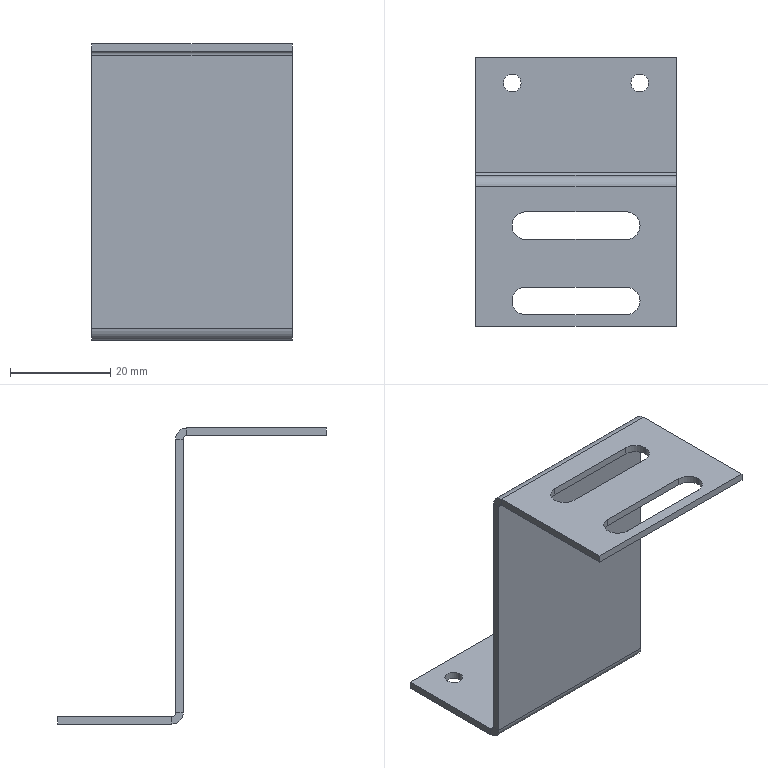Part | SolidWorks | features EdgeFlange 2, FlatPattern 1, ICE 1, SMBaseFlange 1, SheetMetal 1 | 1 solid | 36 faces | box 40 x 53.5 x 59 mm | volume 6153 mm3 | plane 22 | cylinder 14 | commonest cylinder face diameters 5.5 x6 3.5 x4 1.473 x2 4.473 x2
STEP:
#1=CARTESIAN_POINT('',(-14.45,33.5,-57.5));
#2=VERTEX_POINT('',#1);
#3=CARTESIAN_POINT('',(-10.95,33.5,-57.5));
#4=VERTEX_POINT('',#3);
#5=CARTESIAN_POINT('',(-12.7,33.5,-57.5));
#6=DIRECTION('',(0.,0.,1.));
#7=DIRECTION('',(1.,0.,0.));
#8=AXIS2_PLACEMENT_3D('',#5,#6,#7);
#9=CIRCLE('',#8,1.75);
#10=EDGE_CURVE('',#2,#4,#9,.T.);
#11=ORIENTED_EDGE('',*,*,#10,.T.);
#12=CARTESIAN_POINT('',(-10.95,33.5,-59.));
#13=VERTEX_POINT('',#12);
#14=CARTESIAN_POINT('',(-10.95,33.5,-49.));
#15=DIRECTION('',(0.,0.,-1.));
#16=VECTOR('',#15,1000.);
#17=LINE('',#14,#16);
#18=EDGE_CURVE('',#4,#13,#17,.T.);
#19=ORIENTED_EDGE('',*,*,#18,.T.);
#20=CARTESIAN_POINT('',(-14.45,33.5,-59.));
#21=VERTEX_POINT('',#20);
#22=CARTESIAN_POINT('',(-12.7,33.5,-59.));
#23=DIRECTION('',(0.,0.,-1.));
#24=DIRECTION('',(-1.,0.,0.));
#25=AXIS2_PLACEMENT_3D('',#22,#23,#24);
#26=CIRCLE('',#25,1.75);
#27=EDGE_CURVE('',#13,#21,#26,.T.);
#28=ORIENTED_EDGE('',*,*,#27,.T.);
#29=CARTESIAN_POINT('',(-14.45,33.5,-49.));
#30=DIRECTION('',(0.,0.,-1.));
#31=VECTOR('',#30,1000.);
#32=LINE('',#29,#31);
#33=EDGE_CURVE('',#2,#21,#32,.T.);
#34=ORIENTED_EDGE('',*,*,#33,.F.);
#35=EDGE_LOOP('',(#11,#19,#28,#34));
#36=FACE_OUTER_BOUND('',#35,.T.);
#37=CARTESIAN_POINT('',(-12.7,33.5,-49.));
#38=DIRECTION('',(0.,0.,-1.));
#39=DIRECTION('',(-1.,0.,0.));
#40=AXIS2_PLACEMENT_3D('',#37,#38,#39);
#41=CYLINDRICAL_SURFACE('',#40,1.75);
#42=ADVANCED_FACE('',(#36),#41,.F.);
#43=CARTESIAN_POINT('',(10.95,33.5,-57.5));
#44=VERTEX_POINT('',#43);
#45=CARTESIAN_POINT('',(14.45,33.5,-57.5));
#46=VERTEX_POINT('',#45);
#47=CARTESIAN_POINT('',(12.7,33.5,-57.5));
#48=DIRECTION('',(0.,0.,1.));
#49=DIRECTION('',(1.,0.,0.));
#50=AXIS2_PLACEMENT_3D('',#47,#48,#49);
#51=CIRCLE('',#50,1.75);
#52=EDGE_CURVE('',#44,#46,#51,.T.);
#53=ORIENTED_EDGE('',*,*,#52,.T.);
#54=CARTESIAN_POINT('',(14.45,33.5,-59.));
#55=VERTEX_POINT('',#54);
#56=CARTESIAN_POINT('',(14.45,33.5,-49.));
#57=DIRECTION('',(0.,0.,-1.));
#58=VECTOR('',#57,1000.);
#59=LINE('',#56,#58);
#60=EDGE_CURVE('',#46,#55,#59,.T.);
#61=ORIENTED_EDGE('',*,*,#60,.T.);
#62=CARTESIAN_POINT('',(10.95,33.5,-59.));
#63=VERTEX_POINT('',#62);
#64=CARTESIAN_POINT('',(12.7,33.5,-59.));
#65=DIRECTION('',(0.,0.,-1.));
#66=DIRECTION('',(-1.,0.,0.));
#67=AXIS2_PLACEMENT_3D('',#64,#65,#66);
#68=CIRCLE('',#67,1.75);
#69=EDGE_CURVE('',#55,#63,#68,.T.);
#70=ORIENTED_EDGE('',*,*,#69,.T.);
#71=CARTESIAN_POINT('',(10.95,33.5,-49.));
#72=DIRECTION('',(0.,0.,-1.));
#73=VECTOR('',#72,1000.);
#74=LINE('',#71,#73);
#75=EDGE_CURVE('',#44,#63,#74,.T.);
#76=ORIENTED_EDGE('',*,*,#75,.F.);
#77=EDGE_LOOP('',(#53,#61,#70,#76));
#78=FACE_OUTER_BOUND('',#77,.T.);
#79=CARTESIAN_POINT('',(12.7,33.5,-49.));
#80=DIRECTION('',(0.,0.,-1.));
#81=DIRECTION('',(-1.,0.,0.));
#82=AXIS2_PLACEMENT_3D('',#79,#80,#81);
#83=CYLINDRICAL_SURFACE('',#82,1.75);
#84=ADVANCED_FACE('',(#78),#83,.F.);
#85=CARTESIAN_POINT('',(12.75,-10.,-1.5));
#86=VERTEX_POINT('',#85);
#87=CARTESIAN_POINT('',(10.,-7.25,-1.5));
#88=VERTEX_POINT('',#87);
#89=CARTESIAN_POINT('',(10.,-10.,-1.5));
#90=DIRECTION('',(0.,0.,1.));
#91=DIRECTION('',(1.,0.,0.));
#92=AXIS2_PLACEMENT_3D('',#89,#90,#91);
#93=CIRCLE('',#92,2.75);
#94=EDGE_CURVE('',#86,#88,#93,.T.);
#95=ORIENTED_EDGE('',*,*,#94,.F.);
#96=CARTESIAN_POINT('',(12.75,-10.,0.));
#97=VERTEX_POINT('',#96);
#98=CARTESIAN_POINT('',(12.75,-10.,-1.5));
#99=DIRECTION('',(0.,0.,1.));
#100=VECTOR('',#99,1000.);
#101=LINE('',#98,#100);
#102=EDGE_CURVE('',#86,#97,#101,.T.);
#103=ORIENTED_EDGE('',*,*,#102,.T.);
#104=CARTESIAN_POINT('',(10.,-7.25,0.));
#105=VERTEX_POINT('',#104);
#106=CARTESIAN_POINT('',(10.,-10.,0.));
#107=DIRECTION('',(0.,0.,1.));
#108=DIRECTION('',(1.,0.,0.));
#109=AXIS2_PLACEMENT_3D('',#106,#107,#108);
#110=CIRCLE('',#109,2.75);
#111=EDGE_CURVE('',#97,#105,#110,.T.);
#112=ORIENTED_EDGE('',*,*,#111,.T.);
#113=CARTESIAN_POINT('',(10.,-7.25,-1.5));
#114=DIRECTION('',(0.,0.,1.));
#115=VECTOR('',#114,1000.);
#116=LINE('',#113,#115);
#117=EDGE_CURVE('',#88,#105,#116,.T.);
#118=ORIENTED_EDGE('',*,*,#117,.F.);
#119=EDGE_LOOP('',(#95,#103,#112,#118));
#120=FACE_OUTER_BOUND('',#119,.T.);
#121=CARTESIAN_POINT('',(10.,-10.,-1.5));
#122=DIRECTION('',(0.,0.,1.));
#123=DIRECTION('',(1.,0.,0.));
#124=AXIS2_PLACEMENT_3D('',#121,#122,#123);
#125=CYLINDRICAL_SURFACE('',#124,2.75);
#126=ADVANCED_FACE('',(#120),#125,.F.);
#127=CARTESIAN_POINT('',(12.75,5.,-1.5));
#128=VERTEX_POINT('',#127);
#129=CARTESIAN_POINT('',(10.,7.75,-1.5));
#130=VERTEX_POINT('',#129);
#131=CARTESIAN_POINT('',(10.,5.,-1.5));
#132=DIRECTION('',(0.,0.,1.));
#133=DIRECTION('',(1.,0.,0.));
#134=AXIS2_PLACEMENT_3D('',#131,#132,#133);
#135=CIRCLE('',#134,2.75);
#136=EDGE_CURVE('',#128,#130,#135,.T.);
#137=ORIENTED_EDGE('',*,*,#136,.F.);
#138=CARTESIAN_POINT('',(12.75,5.,0.));
#139=VERTEX_POINT('',#138);
#140=CARTESIAN_POINT('',(12.75,5.,-1.5));
#141=DIRECTION('',(0.,0.,1.));
#142=VECTOR('',#141,1000.);
#143=LINE('',#140,#142);
#144=EDGE_CURVE('',#128,#139,#143,.T.);
#145=ORIENTED_EDGE('',*,*,#144,.T.);
#146=CARTESIAN_POINT('',(10.,7.75,0.));
#147=VERTEX_POINT('',#146);
#148=CARTESIAN_POINT('',(10.,5.,0.));
#149=DIRECTION('',(0.,0.,1.));
#150=DIRECTION('',(1.,0.,0.));
#151=AXIS2_PLACEMENT_3D('',#148,#149,#150);
#152=CIRCLE('',#151,2.75);
#153=EDGE_CURVE('',#139,#147,#152,.T.);
#154=ORIENTED_EDGE('',*,*,#153,.T.);
#155=CARTESIAN_POINT('',(10.,7.75,-1.5));
#156=DIRECTION('',(0.,0.,1.));
#157=VECTOR('',#156,1000.);
#158=LINE('',#155,#157);
#159=EDGE_CURVE('',#130,#147,#158,.T.);
#160=ORIENTED_EDGE('',*,*,#159,.F.);
#161=EDGE_LOOP('',(#137,#145,#154,#160));
#162=FACE_OUTER_BOUND('',#161,.T.);
#163=CARTESIAN_POINT('',(10.,5.,-1.5));
#164=DIRECTION('',(0.,0.,1.));
#165=DIRECTION('',(1.,0.,0.));
#166=AXIS2_PLACEMENT_3D('',#163,#164,#165);
#167=CYLINDRICAL_SURFACE('',#166,2.75);
#168=ADVANCED_FACE('',(#162),#167,.F.);
#169=CARTESIAN_POINT('',(-20.,15.,-2.237));
#170=VERTEX_POINT('',#169);
#171=CARTESIAN_POINT('',(-20.,15.,-56.763));
#172=VERTEX_POINT('',#171);
#173=CARTESIAN_POINT('',(-20.,15.,-59.));
#174=DIRECTION('',(0.,0.,-1.));
#175=VECTOR('',#174,1000.);
#176=LINE('',#173,#175);
#177=EDGE_CURVE('',#170,#172,#176,.T.);
#178=ORIENTED_EDGE('',*,*,#177,.T.);
#179=CARTESIAN_POINT('',(-20.,13.5,-56.763));
#180=VERTEX_POINT('',#179);
#181=CARTESIAN_POINT('',(-20.,15.,-56.763));
#182=DIRECTION('',(0.,-1.,0.));
#183=VECTOR('',#182,1000.);
#184=LINE('',#181,#183);
#185=EDGE_CURVE('',#172,#180,#184,.T.);
#186=ORIENTED_EDGE('',*,*,#185,.T.);
#187=CARTESIAN_POINT('',(-20.,13.5,-2.237));
#188=VERTEX_POINT('',#187);
#189=CARTESIAN_POINT('',(-20.,13.5,0.));
#190=DIRECTION('',(0.,0.,-1.));
#191=VECTOR('',#190,1000.);
#192=LINE('',#189,#191);
#193=EDGE_CURVE('',#188,#180,#192,.T.);
#194=ORIENTED_EDGE('',*,*,#193,.F.);
#195=CARTESIAN_POINT('',(-20.,15.,-2.237));
#196=DIRECTION('',(0.,1.,0.));
#197=VECTOR('',#196,1000.);
#198=LINE('',#195,#197);
#199=EDGE_CURVE('',#188,#170,#198,.T.);
#200=ORIENTED_EDGE('',*,*,#199,.T.);
#201=EDGE_LOOP('',(#178,#186,#194,#200));
#202=FACE_OUTER_BOUND('',#201,.T.);
#203=CARTESIAN_POINT('',(-20.,15.,-59.));
#204=DIRECTION('',(-1.,0.,0.));
#205=DIRECTION('',(0.,0.,1.));
#206=AXIS2_PLACEMENT_3D('',#203,#204,#205);
#207=PLANE('',#206);
#208=ADVANCED_FACE('',(#202),#207,.T.);
#209=CARTESIAN_POINT('',(20.,15.,-56.763));
#210=VERTEX_POINT('',#209);
#211=CARTESIAN_POINT('',(20.,15.,-2.237));
#212=VERTEX_POINT('',#211);
#213=CARTESIAN_POINT('',(20.,15.,-1.5));
#214=DIRECTION('',(0.,0.,1.));
#215=VECTOR('',#214,1000.);
#216=LINE('',#213,#215);
#217=EDGE_CURVE('',#210,#212,#216,.T.);
#218=ORIENTED_EDGE('',*,*,#217,.F.);
#219=CARTESIAN_POINT('',(-20.,15.,-56.763));
#220=DIRECTION('',(1.,0.,0.));
#221=VECTOR('',#220,1000.);
#222=LINE('',#219,#221);
#223=EDGE_CURVE('',#172,#210,#222,.T.);
#224=ORIENTED_EDGE('',*,*,#223,.F.);
#225=ORIENTED_EDGE('',*,*,#177,.F.);
#226=CARTESIAN_POINT('',(0.,15.,-2.237));
#227=DIRECTION('',(1.,0.,0.));
#228=VECTOR('',#227,1000.);
#229=LINE('',#226,#228);
#230=EDGE_CURVE('',#170,#212,#229,.T.);
#231=ORIENTED_EDGE('',*,*,#230,.T.);
#232=EDGE_LOOP('',(#218,#224,#225,#231));
#233=FACE_OUTER_BOUND('',#232,.T.);
#234=CARTESIAN_POINT('',(0.,15.,0.));
#235=DIRECTION('',(0.,1.,0.));
#236=DIRECTION('',(0.,0.,1.));
#237=AXIS2_PLACEMENT_3D('',#234,#235,#236);
#238=PLANE('',#237);
#239=ADVANCED_FACE('',(#233),#238,.T.);
#240=CARTESIAN_POINT('',(20.,13.5,-56.763));
#241=VERTEX_POINT('',#240);
#242=CARTESIAN_POINT('',(-20.,13.5,-56.763));
#243=DIRECTION('',(1.,0.,0.));
#244=VECTOR('',#243,1000.);
#245=LINE('',#242,#244);
#246=EDGE_CURVE('',#180,#241,#245,.T.);
#247=ORIENTED_EDGE('',*,*,#246,.T.);
#248=CARTESIAN_POINT('',(20.,13.5,-2.237));
#249=VERTEX_POINT('',#248);
#250=CARTESIAN_POINT('',(20.,13.5,0.));
#251=DIRECTION('',(0.,0.,1.));
#252=VECTOR('',#251,1000.);
#253=LINE('',#250,#252);
#254=EDGE_CURVE('',#241,#249,#253,.T.);
#255=ORIENTED_EDGE('',*,*,#254,.T.);
#256=CARTESIAN_POINT('',(-20.,13.5,-2.237));
#257=DIRECTION('',(1.,0.,0.));
#258=VECTOR('',#257,1000.);
#259=LINE('',#256,#258);
#260=EDGE_CURVE('',#188,#249,#259,.T.);
#261=ORIENTED_EDGE('',*,*,#260,.F.);
#262=ORIENTED_EDGE('',*,*,#193,.T.);
#263=EDGE_LOOP('',(#247,#255,#261,#262));
#264=FACE_OUTER_BOUND('',#263,.T.);
#265=CARTESIAN_POINT('',(0.,13.5,0.));
#266=DIRECTION('',(0.,1.,0.));
#267=DIRECTION('',(0.,0.,1.));
#268=AXIS2_PLACEMENT_3D('',#265,#266,#267);
#269=PLANE('',#268);
#270=ADVANCED_FACE('',(#264),#269,.F.);
#271=CARTESIAN_POINT('',(20.,-15.,-1.5));
#272=VERTEX_POINT('',#271);
#273=CARTESIAN_POINT('',(20.,12.763,-1.5));
#274=VERTEX_POINT('',#273);
#275=CARTESIAN_POINT('',(20.,15.,-1.5));
#276=DIRECTION('',(0.,1.,0.));
#277=VECTOR('',#276,1000.);
#278=LINE('',#275,#277);
#279=EDGE_CURVE('',#272,#274,#278,.T.);
#280=ORIENTED_EDGE('',*,*,#279,.T.);
#281=CARTESIAN_POINT('',(20.,12.763,0.));
#282=VERTEX_POINT('',#281);
#283=CARTESIAN_POINT('',(20.,12.763,-1.5));
#284=DIRECTION('',(0.,0.,1.));
#285=VECTOR('',#284,1000.);
#286=LINE('',#283,#285);
#287=EDGE_CURVE('',#274,#282,#286,.T.);
#288=ORIENTED_EDGE('',*,*,#287,.T.);
#289=CARTESIAN_POINT('',(20.,-15.,0.));
#290=VERTEX_POINT('',#289);
#291=CARTESIAN_POINT('',(20.,15.,0.));
#292=DIRECTION('',(0.,1.,0.));
#293=VECTOR('',#292,1000.);
#294=LINE('',#291,#293);
#295=EDGE_CURVE('',#290,#282,#294,.T.);
#296=ORIENTED_EDGE('',*,*,#295,.F.);
#297=CARTESIAN_POINT('',(20.,-15.,-1.5));
#298=DIRECTION('',(0.,0.,1.));
#299=VECTOR('',#298,1000.);
#300=LINE('',#297,#299);
#301=EDGE_CURVE('',#272,#290,#300,.T.);
#302=ORIENTED_EDGE('',*,*,#301,.F.);
#303=EDGE_LOOP('',(#280,#288,#296,#302));
#304=FACE_OUTER_BOUND('',#303,.T.);
#305=CARTESIAN_POINT('',(20.,15.,-1.5));
#306=DIRECTION('',(1.,0.,0.));
#307=DIRECTION('',(0.,0.,-1.));
#308=AXIS2_PLACEMENT_3D('',#305,#306,#307);
#309=PLANE('',#308);
#310=ADVANCED_FACE('',(#304),#309,.T.);
#311=CARTESIAN_POINT('',(-10.,2.25,-1.5));
#312=VERTEX_POINT('',#311);
#313=CARTESIAN_POINT('',(10.,2.25,-1.5));
#314=VERTEX_POINT('',#313);
#315=CARTESIAN_POINT('',(10.,2.25,-1.5));
#316=DIRECTION('',(1.,0.,0.));
#317=VECTOR('',#316,1000.);
#318=LINE('',#315,#317);
#319=EDGE_CURVE('',#312,#314,#318,.T.);
#320=ORIENTED_EDGE('',*,*,#319,.T.);
#321=CARTESIAN_POINT('',(10.,5.,-1.5));
#322=DIRECTION('',(0.,0.,1.));
#323=DIRECTION('',(1.,0.,0.));
#324=AXIS2_PLACEMENT_3D('',#321,#322,#323);
#325=CIRCLE('',#324,2.75);
#326=EDGE_CURVE('',#314,#128,#325,.T.);
#327=ORIENTED_EDGE('',*,*,#326,.T.);
#328=ORIENTED_EDGE('',*,*,#136,.T.);
#329=CARTESIAN_POINT('',(-10.,7.75,-1.5));
#330=VERTEX_POINT('',#329);
#331=CARTESIAN_POINT('',(10.,7.75,-1.5));
#332=DIRECTION('',(-1.,0.,0.));
#333=VECTOR('',#332,1000.);
#334=LINE('',#331,#333);
#335=EDGE_CURVE('',#130,#330,#334,.T.);
#336=ORIENTED_EDGE('',*,*,#335,.T.);
#337=CARTESIAN_POINT('',(-10.,5.,-1.5));
#338=DIRECTION('',(0.,0.,1.));
#339=DIRECTION('',(1.,0.,0.));
#340=AXIS2_PLACEMENT_3D('',#337,#338,#339);
#341=CIRCLE('',#340,2.75);
#342=EDGE_CURVE('',#330,#312,#341,.T.);
#343=ORIENTED_EDGE('',*,*,#342,.T.);
#344=EDGE_LOOP('',(#320,#327,#328,#336,#343));
#345=FACE_BOUND('',#344,.T.);
#346=CARTESIAN_POINT('',(-10.,-12.75,-1.5));
#347=VERTEX_POINT('',#346);
#348=CARTESIAN_POINT('',(10.,-12.75,-1.5));
#349=VERTEX_POINT('',#348);
#350=CARTESIAN_POINT('',(10.,-12.75,-1.5));
#351=DIRECTION('',(1.,0.,0.));
#352=VECTOR('',#351,1000.);
#353=LINE('',#350,#352);
#354=EDGE_CURVE('',#347,#349,#353,.T.);
#355=ORIENTED_EDGE('',*,*,#354,.T.);
#356=CARTESIAN_POINT('',(10.,-10.,-1.5));
#357=DIRECTION('',(0.,0.,1.));
#358=DIRECTION('',(1.,0.,0.));
#359=AXIS2_PLACEMENT_3D('',#356,#357,#358);
#360=CIRCLE('',#359,2.75);
#361=EDGE_CURVE('',#349,#86,#360,.T.);
#362=ORIENTED_EDGE('',*,*,#361,.T.);
#363=ORIENTED_EDGE('',*,*,#94,.T.);
#364=CARTESIAN_POINT('',(-10.,-7.25,-1.5));
#365=VERTEX_POINT('',#364);
#366=CARTESIAN_POINT('',(10.,-7.25,-1.5));
#367=DIRECTION('',(-1.,0.,0.));
#368=VECTOR('',#367,1000.);
#369=LINE('',#366,#368);
#370=EDGE_CURVE('',#88,#365,#369,.T.);
#371=ORIENTED_EDGE('',*,*,#370,.T.);
#372=CARTESIAN_POINT('',(-10.,-10.,-1.5));
#373=DIRECTION('',(0.,0.,1.));
#374=DIRECTION('',(1.,0.,0.));
#375=AXIS2_PLACEMENT_3D('',#372,#373,#374);
#376=CIRCLE('',#375,2.75);
#377=EDGE_CURVE('',#365,#347,#376,.T.);
#378=ORIENTED_EDGE('',*,*,#377,.T.);
#379=EDGE_LOOP('',(#355,#362,#363,#371,#378));
#380=FACE_BOUND('',#379,.T.);
#381=CARTESIAN_POINT('',(-20.,12.763,-1.5));
#382=VERTEX_POINT('',#381);
#383=CARTESIAN_POINT('',(20.,12.763,-1.5));
#384=DIRECTION('',(-1.,0.,0.));
#385=VECTOR('',#384,1000.);
#386=LINE('',#383,#385);
#387=EDGE_CURVE('',#274,#382,#386,.T.);
#388=ORIENTED_EDGE('',*,*,#387,.F.);
#389=ORIENTED_EDGE('',*,*,#279,.F.);
#390=CARTESIAN_POINT('',(-20.,-15.,-1.5));
#391=VERTEX_POINT('',#390);
#392=CARTESIAN_POINT('',(-20.,-15.,-1.5));
#393=DIRECTION('',(1.,0.,0.));
#394=VECTOR('',#393,1000.);
#395=LINE('',#392,#394);
#396=EDGE_CURVE('',#391,#272,#395,.T.);
#397=ORIENTED_EDGE('',*,*,#396,.F.);
#398=CARTESIAN_POINT('',(-20.,15.,-1.5));
#399=DIRECTION('',(0.,-1.,0.));
#400=VECTOR('',#399,1000.);
#401=LINE('',#398,#400);
#402=EDGE_CURVE('',#382,#391,#401,.T.);
#403=ORIENTED_EDGE('',*,*,#402,.F.);
#404=EDGE_LOOP('',(#388,#389,#397,#403));
#405=FACE_OUTER_BOUND('',#404,.T.);
#406=CARTESIAN_POINT('',(0.,0.,-1.5));
#407=DIRECTION('',(0.,0.,1.));
#408=DIRECTION('',(1.,0.,0.));
#409=AXIS2_PLACEMENT_3D('',#406,#407,#408);
#410=PLANE('',#409);
#411=ADVANCED_FACE('',(#345,#380,#405),#410,.F.);
#412=CARTESIAN_POINT('',(10.,2.25,0.));
#413=VERTEX_POINT('',#412);
#414=CARTESIAN_POINT('',(10.,5.,0.));
#415=DIRECTION('',(0.,0.,1.));
#416=DIRECTION('',(1.,0.,0.));
#417=AXIS2_PLACEMENT_3D('',#414,#415,#416);
#418=CIRCLE('',#417,2.75);
#419=EDGE_CURVE('',#413,#139,#418,.T.);
#420=ORIENTED_EDGE('',*,*,#419,.F.);
#421=CARTESIAN_POINT('',(-10.,2.25,0.));
#422=VERTEX_POINT('',#421);
#423=CARTESIAN_POINT('',(10.,2.25,0.));
#424=DIRECTION('',(1.,0.,0.));
#425=VECTOR('',#424,1000.);
#426=LINE('',#423,#425);
#427=EDGE_CURVE('',#422,#413,#426,.T.);
#428=ORIENTED_EDGE('',*,*,#427,.F.);
#429=CARTESIAN_POINT('',(-10.,7.75,0.));
#430=VERTEX_POINT('',#429);
#431=CARTESIAN_POINT('',(-10.,5.,0.));
#432=DIRECTION('',(0.,0.,1.));
#433=DIRECTION('',(1.,0.,0.));
#434=AXIS2_PLACEMENT_3D('',#431,#432,#433);
#435=CIRCLE('',#434,2.75);
#436=EDGE_CURVE('',#430,#422,#435,.T.);
#437=ORIENTED_EDGE('',*,*,#436,.F.);
#438=CARTESIAN_POINT('',(10.,7.75,0.));
#439=DIRECTION('',(-1.,0.,0.));
#440=VECTOR('',#439,1000.);
#441=LINE('',#438,#440);
#442=EDGE_CURVE('',#147,#430,#441,.T.);
#443=ORIENTED_EDGE('',*,*,#442,.F.);
#444=ORIENTED_EDGE('',*,*,#153,.F.);
#445=EDGE_LOOP('',(#420,#428,#437,#443,#444));
#446=FACE_BOUND('',#445,.T.);
#447=CARTESIAN_POINT('',(10.,-12.75,0.));
#448=VERTEX_POINT('',#447);
#449=CARTESIAN_POINT('',(10.,-10.,0.));
#450=DIRECTION('',(0.,0.,1.));
#451=DIRECTION('',(1.,0.,0.));
#452=AXIS2_PLACEMENT_3D('',#449,#450,#451);
#453=CIRCLE('',#452,2.75);
#454=EDGE_CURVE('',#448,#97,#453,.T.);
#455=ORIENTED_EDGE('',*,*,#454,.F.);
#456=CARTESIAN_POINT('',(-10.,-12.75,0.));
#457=VERTEX_POINT('',#456);
#458=CARTESIAN_POINT('',(10.,-12.75,0.));
#459=DIRECTION('',(1.,0.,0.));
#460=VECTOR('',#459,1000.);
#461=LINE('',#458,#460);
#462=EDGE_CURVE('',#457,#448,#461,.T.);
#463=ORIENTED_EDGE('',*,*,#462,.F.);
#464=CARTESIAN_POINT('',(-10.,-7.25,0.));
#465=VERTEX_POINT('',#464);
#466=CARTESIAN_POINT('',(-10.,-10.,0.));
#467=DIRECTION('',(0.,0.,1.));
#468=DIRECTION('',(1.,0.,0.));
#469=AXIS2_PLACEMENT_3D('',#466,#467,#468);
#470=CIRCLE('',#469,2.75);
#471=EDGE_CURVE('',#465,#457,#470,.T.);
#472=ORIENTED_EDGE('',*,*,#471,.F.);
#473=CARTESIAN_POINT('',(10.,-7.25,0.));
#474=DIRECTION('',(-1.,0.,0.));
#475=VECTOR('',#474,1000.);
#476=LINE('',#473,#475);
#477=EDGE_CURVE('',#105,#465,#476,.T.);
#478=ORIENTED_EDGE('',*,*,#477,.F.);
#479=ORIENTED_EDGE('',*,*,#111,.F.);
#480=EDGE_LOOP('',(#455,#463,#472,#478,#479));
#481=FACE_BOUND('',#480,.T.);
#482=ORIENTED_EDGE('',*,*,#295,.T.);
#483=CARTESIAN_POINT('',(-20.,12.763,0.));
#484=VERTEX_POINT('',#483);
#485=CARTESIAN_POINT('',(20.,12.763,0.));
#486=DIRECTION('',(-1.,0.,0.));
#487=VECTOR('',#486,1000.);
#488=LINE('',#485,#487);
#489=EDGE_CURVE('',#282,#484,#488,.T.);
#490=ORIENTED_EDGE('',*,*,#489,.T.);
#491=CARTESIAN_POINT('',(-20.,-15.,0.));
#492=VERTEX_POINT('',#491);
#493=CARTESIAN_POINT('',(-20.,15.,0.));
#494=DIRECTION('',(0.,-1.,0.));
#495=VECTOR('',#494,1000.);
#496=LINE('',#493,#495);
#497=EDGE_CURVE('',#484,#492,#496,.T.);
#498=ORIENTED_EDGE('',*,*,#497,.T.);
#499=CARTESIAN_POINT('',(-20.,-15.,0.));
#500=DIRECTION('',(1.,0.,0.));
#501=VECTOR('',#500,1000.);
#502=LINE('',#499,#501);
#503=EDGE_CURVE('',#492,#290,#502,.T.);
#504=ORIENTED_EDGE('',*,*,#503,.T.);
#505=EDGE_LOOP('',(#482,#490,#498,#504));
#506=FACE_OUTER_BOUND('',#505,.T.);
#507=CARTESIAN_POINT('',(0.,0.,0.));
#508=DIRECTION('',(0.,0.,1.));
#509=DIRECTION('',(1.,0.,0.));
#510=AXIS2_PLACEMENT_3D('',#507,#508,#509);
#511=PLANE('',#510);
#512=ADVANCED_FACE('',(#446,#481,#506),#511,.T.);
#513=ORIENTED_EDGE('',*,*,#503,.F.);
#514=CARTESIAN_POINT('',(-20.,-15.,-1.5));
#515=DIRECTION('',(0.,0.,1.));
#516=VECTOR('',#515,1000.);
#517=LINE('',#514,#516);
#518=EDGE_CURVE('',#391,#492,#517,.T.);
#519=ORIENTED_EDGE('',*,*,#518,.F.);
#520=ORIENTED_EDGE('',*,*,#396,.T.);
#521=ORIENTED_EDGE('',*,*,#301,.T.);
#522=EDGE_LOOP('',(#513,#519,#520,#521));
#523=FACE_OUTER_BOUND('',#522,.T.);
#524=CARTESIAN_POINT('',(-20.,-15.,-1.5));
#525=DIRECTION('',(0.,-1.,0.));
#526=DIRECTION('',(0.,0.,-1.));
#527=AXIS2_PLACEMENT_3D('',#524,#525,#526);
#528=PLANE('',#527);
#529=ADVANCED_FACE('',(#523),#528,.T.);
#530=CARTESIAN_POINT('',(-20.,12.763,-1.5));
#531=DIRECTION('',(0.,0.,1.));
#532=VECTOR('',#531,1000.);
#533=LINE('',#530,#532);
#534=EDGE_CURVE('',#382,#484,#533,.T.);
#535=ORIENTED_EDGE('',*,*,#534,.F.);
#536=ORIENTED_EDGE('',*,*,#402,.T.);
#537=ORIENTED_EDGE('',*,*,#518,.T.);
#538=ORIENTED_EDGE('',*,*,#497,.F.);
#539=EDGE_LOOP('',(#535,#536,#537,#538));
#540=FACE_OUTER_BOUND('',#539,.T.);
#541=CARTESIAN_POINT('',(-20.,15.,-1.5));
#542=DIRECTION('',(-1.,0.,0.));
#543=DIRECTION('',(0.,0.,1.));
#544=AXIS2_PLACEMENT_3D('',#541,#542,#543);
#545=PLANE('',#544);
#546=ADVANCED_FACE('',(#540),#545,.T.);
#547=ORIENTED_EDGE('',*,*,#144,.F.);
#548=ORIENTED_EDGE('',*,*,#326,.F.);
#549=CARTESIAN_POINT('',(10.,2.25,-1.5));
#550=DIRECTION('',(0.,0.,1.));
#551=VECTOR('',#550,1000.);
#552=LINE('',#549,#551);
#553=EDGE_CURVE('',#314,#413,#552,.T.);
#554=ORIENTED_EDGE('',*,*,#553,.T.);
#555=ORIENTED_EDGE('',*,*,#419,.T.);
#556=EDGE_LOOP('',(#547,#548,#554,#555));
#557=FACE_OUTER_BOUND('',#556,.T.);
#558=CARTESIAN_POINT('',(10.,5.,-1.5));
#559=DIRECTION('',(0.,0.,1.));
#560=DIRECTION('',(1.,0.,0.));
#561=AXIS2_PLACEMENT_3D('',#558,#559,#560);
#562=CYLINDRICAL_SURFACE('',#561,2.75);
#563=ADVANCED_FACE('',(#557),#562,.F.);
#564=ORIENTED_EDGE('',*,*,#427,.T.);
#565=ORIENTED_EDGE('',*,*,#553,.F.);
#566=ORIENTED_EDGE('',*,*,#319,.F.);
#567=CARTESIAN_POINT('',(-10.,2.25,-1.5));
#568=DIRECTION('',(0.,0.,1.));
#569=VECTOR('',#568,1000.);
#570=LINE('',#567,#569);
#571=EDGE_CURVE('',#312,#422,#570,.T.);
#572=ORIENTED_EDGE('',*,*,#571,.T.);
#573=EDGE_LOOP('',(#564,#565,#566,#572));
#574=FACE_OUTER_BOUND('',#573,.T.);
#575=CARTESIAN_POINT('',(10.,2.25,-1.5));
#576=DIRECTION('',(0.,-1.,0.));
#577=DIRECTION('',(0.,0.,-1.));
#578=AXIS2_PLACEMENT_3D('',#575,#576,#577);
#579=PLANE('',#578);
#580=ADVANCED_FACE('',(#574),#579,.F.);
#581=ORIENTED_EDGE('',*,*,#436,.T.);
#582=ORIENTED_EDGE('',*,*,#571,.F.);
#583=ORIENTED_EDGE('',*,*,#342,.F.);
#584=CARTESIAN_POINT('',(-10.,7.75,-1.5));
#585=DIRECTION('',(0.,0.,1.));
#586=VECTOR('',#585,1000.);
#587=LINE('',#584,#586);
#588=EDGE_CURVE('',#330,#430,#587,.T.);
#589=ORIENTED_EDGE('',*,*,#588,.T.);
#590=EDGE_LOOP('',(#581,#582,#583,#589));
#591=FACE_OUTER_BOUND('',#590,.T.);
#592=CARTESIAN_POINT('',(-10.,5.,-1.5));
#593=DIRECTION('',(0.,0.,1.));
#594=DIRECTION('',(1.,0.,0.));
#595=AXIS2_PLACEMENT_3D('',#592,#593,#594);
#596=CYLINDRICAL_SURFACE('',#595,2.75);
#597=ADVANCED_FACE('',(#591),#596,.F.);
#598=ORIENTED_EDGE('',*,*,#442,.T.);
#599=ORIENTED_EDGE('',*,*,#588,.F.);
#600=ORIENTED_EDGE('',*,*,#335,.F.);
#601=ORIENTED_EDGE('',*,*,#159,.T.);
#602=EDGE_LOOP('',(#598,#599,#600,#601));
#603=FACE_OUTER_BOUND('',#602,.T.);
#604=CARTESIAN_POINT('',(10.,7.75,-1.5));
#605=DIRECTION('',(0.,1.,0.));
#606=DIRECTION('',(0.,0.,1.));
#607=AXIS2_PLACEMENT_3D('',#604,#605,#606);
#608=PLANE('',#607);
#609=ADVANCED_FACE('',(#603),#608,.F.);
#610=ORIENTED_EDGE('',*,*,#102,.F.);
#611=ORIENTED_EDGE('',*,*,#361,.F.);
#612=CARTESIAN_POINT('',(10.,-12.75,-1.5));
#613=DIRECTION('',(0.,0.,1.));
#614=VECTOR('',#613,1000.);
#615=LINE('',#612,#614);
#616=EDGE_CURVE('',#349,#448,#615,.T.);
#617=ORIENTED_EDGE('',*,*,#616,.T.);
#618=ORIENTED_EDGE('',*,*,#454,.T.);
#619=EDGE_LOOP('',(#610,#611,#617,#618));
#620=FACE_OUTER_BOUND('',#619,.T.);
#621=CARTESIAN_POINT('',(10.,-10.,-1.5));
#622=DIRECTION('',(0.,0.,1.));
#623=DIRECTION('',(1.,0.,0.));
#624=AXIS2_PLACEMENT_3D('',#621,#622,#623);
#625=CYLINDRICAL_SURFACE('',#624,2.75);
#626=ADVANCED_FACE('',(#620),#625,.F.);
#627=ORIENTED_EDGE('',*,*,#462,.T.);
#628=ORIENTED_EDGE('',*,*,#616,.F.);
#629=ORIENTED_EDGE('',*,*,#354,.F.);
#630=CARTESIAN_POINT('',(-10.,-12.75,-1.5));
#631=DIRECTION('',(0.,0.,1.));
#632=VECTOR('',#631,1000.);
#633=LINE('',#630,#632);
#634=EDGE_CURVE('',#347,#457,#633,.T.);
#635=ORIENTED_EDGE('',*,*,#634,.T.);
#636=EDGE_LOOP('',(#627,#628,#629,#635));
#637=FACE_OUTER_BOUND('',#636,.T.);
#638=CARTESIAN_POINT('',(10.,-12.75,-1.5));
#639=DIRECTION('',(0.,-1.,0.));
#640=DIRECTION('',(0.,0.,-1.));
#641=AXIS2_PLACEMENT_3D('',#638,#639,#640);
#642=PLANE('',#641);
#643=ADVANCED_FACE('',(#637),#642,.F.);
#644=ORIENTED_EDGE('',*,*,#471,.T.);
#645=ORIENTED_EDGE('',*,*,#634,.F.);
#646=ORIENTED_EDGE('',*,*,#377,.F.);
#647=CARTESIAN_POINT('',(-10.,-7.25,-1.5));
#648=DIRECTION('',(0.,0.,1.));
#649=VECTOR('',#648,1000.);
#650=LINE('',#647,#649);
#651=EDGE_CURVE('',#365,#465,#650,.T.);
#652=ORIENTED_EDGE('',*,*,#651,.T.);
#653=EDGE_LOOP('',(#644,#645,#646,#652));
#654=FACE_OUTER_BOUND('',#653,.T.);
#655=CARTESIAN_POINT('',(-10.,-10.,-1.5));
#656=DIRECTION('',(0.,0.,1.));
#657=DIRECTION('',(1.,0.,0.));
#658=AXIS2_PLACEMENT_3D('',#655,#656,#657);
#659=CYLINDRICAL_SURFACE('',#658,2.75);
#660=ADVANCED_FACE('',(#654),#659,.F.);
#661=ORIENTED_EDGE('',*,*,#477,.T.);
#662=ORIENTED_EDGE('',*,*,#651,.F.);
#663=ORIENTED_EDGE('',*,*,#370,.F.);
#664=ORIENTED_EDGE('',*,*,#117,.T.);
#665=EDGE_LOOP('',(#661,#662,#663,#664));
#666=FACE_OUTER_BOUND('',#665,.T.);
#667=CARTESIAN_POINT('',(10.,-7.25,-1.5));
#668=DIRECTION('',(0.,1.,0.));
#669=DIRECTION('',(0.,0.,1.));
#670=AXIS2_PLACEMENT_3D('',#667,#668,#669);
#671=PLANE('',#670);
#672=ADVANCED_FACE('',(#666),#671,.F.);
#673=ORIENTED_EDGE('',*,*,#199,.F.);
#674=CARTESIAN_POINT('',(-20.,12.763,-2.237));
#675=DIRECTION('',(-1.,0.,0.));
#676=DIRECTION('',(0.,0.,-1.));
#677=AXIS2_PLACEMENT_3D('',#674,#675,#676);
#678=CIRCLE('',#677,0.7366);
#679=EDGE_CURVE('',#382,#188,#678,.T.);
#680=ORIENTED_EDGE('',*,*,#679,.F.);
#681=ORIENTED_EDGE('',*,*,#534,.T.);
#682=CARTESIAN_POINT('',(-20.,12.763,-2.237));
#683=DIRECTION('',(-1.,0.,0.));
#684=DIRECTION('',(0.,0.,-1.));
#685=AXIS2_PLACEMENT_3D('',#682,#683,#684);
#686=CIRCLE('',#685,2.237);
#687=EDGE_CURVE('',#484,#170,#686,.T.);
#688=ORIENTED_EDGE('',*,*,#687,.T.);
#689=EDGE_LOOP('',(#673,#680,#681,#688));
#690=FACE_OUTER_BOUND('',#689,.T.);
#691=CARTESIAN_POINT('',(-20.,12.763,-2.237));
#692=DIRECTION('',(-1.,0.,0.));
#693=DIRECTION('',(0.,0.,1.));
#694=AXIS2_PLACEMENT_3D('',#691,#692,#693);
#695=PLANE('',#694);
#696=ADVANCED_FACE('',(#690),#695,.T.);
#697=CARTESIAN_POINT('',(20.,12.763,-2.237));
#698=DIRECTION('',(1.,0.,0.));
#699=DIRECTION('',(0.,0.,-1.));
#700=AXIS2_PLACEMENT_3D('',#697,#698,#699);
#701=CIRCLE('',#700,0.7366);
#702=EDGE_CURVE('',#249,#274,#701,.T.);
#703=ORIENTED_EDGE('',*,*,#702,.F.);
#704=CARTESIAN_POINT('',(20.,13.5,-2.237));
#705=DIRECTION('',(0.,1.,0.));
#706=VECTOR('',#705,1000.);
#707=LINE('',#704,#706);
#708=EDGE_CURVE('',#249,#212,#707,.T.);
#709=ORIENTED_EDGE('',*,*,#708,.T.);
#710=CARTESIAN_POINT('',(20.,12.763,-2.237));
#711=DIRECTION('',(1.,0.,0.));
#712=DIRECTION('',(0.,0.,-1.));
#713=AXIS2_PLACEMENT_3D('',#710,#711,#712);
#714=CIRCLE('',#713,2.237);
#715=EDGE_CURVE('',#212,#282,#714,.T.);
#716=ORIENTED_EDGE('',*,*,#715,.T.);
#717=ORIENTED_EDGE('',*,*,#287,.F.);
#718=EDGE_LOOP('',(#703,#709,#716,#717));
#719=FACE_OUTER_BOUND('',#718,.T.);
#720=CARTESIAN_POINT('',(20.,12.763,-2.237));
#721=DIRECTION('',(-1.,0.,0.));
#722=DIRECTION('',(0.,0.,1.));
#723=AXIS2_PLACEMENT_3D('',#720,#721,#722);
#724=PLANE('',#723);
#725=ADVANCED_FACE('',(#719),#724,.F.);
#726=ORIENTED_EDGE('',*,*,#489,.F.);
#727=ORIENTED_EDGE('',*,*,#715,.F.);
#728=ORIENTED_EDGE('',*,*,#230,.F.);
#729=ORIENTED_EDGE('',*,*,#687,.F.);
#730=EDGE_LOOP('',(#726,#727,#728,#729));
#731=FACE_OUTER_BOUND('',#730,.T.);
#732=CARTESIAN_POINT('',(20.,12.763,-2.237));
#733=DIRECTION('',(1.,0.,0.));
#734=DIRECTION('',(0.,1.,0.));
#735=AXIS2_PLACEMENT_3D('',#732,#733,#734);
#736=CYLINDRICAL_SURFACE('',#735,2.237);
#737=ADVANCED_FACE('',(#731),#736,.T.);
#738=ORIENTED_EDGE('',*,*,#387,.T.);
#739=ORIENTED_EDGE('',*,*,#679,.T.);
#740=ORIENTED_EDGE('',*,*,#260,.T.);
#741=ORIENTED_EDGE('',*,*,#702,.T.);
#742=EDGE_LOOP('',(#738,#739,#740,#741));
#743=FACE_OUTER_BOUND('',#742,.T.);
#744=CARTESIAN_POINT('',(20.,12.763,-2.237));
#745=DIRECTION('',(1.,0.,0.));
#746=DIRECTION('',(0.,1.,0.));
#747=AXIS2_PLACEMENT_3D('',#744,#745,#746);
#748=CYLINDRICAL_SURFACE('',#747,0.7366);
#749=ADVANCED_FACE('',(#743),#748,.F.);
#750=CARTESIAN_POINT('',(20.,15.,-56.763));
#751=DIRECTION('',(0.,-1.,0.));
#752=VECTOR('',#751,1000.);
#753=LINE('',#750,#752);
#754=EDGE_CURVE('',#210,#241,#753,.T.);
#755=ORIENTED_EDGE('',*,*,#754,.F.);
#756=ORIENTED_EDGE('',*,*,#217,.T.);
#757=ORIENTED_EDGE('',*,*,#708,.F.);
#758=ORIENTED_EDGE('',*,*,#254,.F.);
#759=EDGE_LOOP('',(#755,#756,#757,#758));
#760=FACE_OUTER_BOUND('',#759,.T.);
#761=CARTESIAN_POINT('',(20.,15.,-1.5));
#762=DIRECTION('',(1.,0.,0.));
#763=DIRECTION('',(0.,0.,-1.));
#764=AXIS2_PLACEMENT_3D('',#761,#762,#763);
#765=PLANE('',#764);
#766=ADVANCED_FACE('',(#760),#765,.T.);
#767=CARTESIAN_POINT('',(20.,15.737,-57.5));
#768=VERTEX_POINT('',#767);
#769=CARTESIAN_POINT('',(20.,15.737,-59.));
#770=VERTEX_POINT('',#769);
#771=CARTESIAN_POINT('',(20.,15.737,-59.));
#772=DIRECTION('',(0.,0.,-1.));
#773=VECTOR('',#772,1000.);
#774=LINE('',#771,#773);
#775=EDGE_CURVE('',#768,#770,#774,.T.);
#776=ORIENTED_EDGE('',*,*,#775,.F.);
#777=CARTESIAN_POINT('',(20.,15.737,-56.763));
#778=DIRECTION('',(1.,0.,0.));
#779=DIRECTION('',(0.,0.,1.));
#780=AXIS2_PLACEMENT_3D('',#777,#778,#779);
#781=CIRCLE('',#780,0.7366);
#782=EDGE_CURVE('',#210,#768,#781,.T.);
#783=ORIENTED_EDGE('',*,*,#782,.F.);
#784=ORIENTED_EDGE('',*,*,#754,.T.);
#785=CARTESIAN_POINT('',(20.,15.737,-56.763));
#786=DIRECTION('',(1.,0.,0.));
#787=DIRECTION('',(0.,0.,1.));
#788=AXIS2_PLACEMENT_3D('',#785,#786,#787);
#789=CIRCLE('',#788,2.237);
#790=EDGE_CURVE('',#241,#770,#789,.T.);
#791=ORIENTED_EDGE('',*,*,#790,.T.);
#792=EDGE_LOOP('',(#776,#783,#784,#791));
#793=FACE_OUTER_BOUND('',#792,.T.);
#794=CARTESIAN_POINT('',(20.,15.737,-56.763));
#795=DIRECTION('',(1.,0.,0.));
#796=DIRECTION('',(0.,0.,-1.));
#797=AXIS2_PLACEMENT_3D('',#794,#795,#796);
#798=PLANE('',#797);
#799=ADVANCED_FACE('',(#793),#798,.T.);
#800=CARTESIAN_POINT('',(-20.,15.737,-57.5));
#801=VERTEX_POINT('',#800);
#802=CARTESIAN_POINT('',(-20.,15.737,-56.763));
#803=DIRECTION('',(-1.,0.,0.));
#804=DIRECTION('',(0.,0.,1.));
#805=AXIS2_PLACEMENT_3D('',#802,#803,#804);
#806=CIRCLE('',#805,0.7366);
#807=EDGE_CURVE('',#801,#172,#806,.T.);
#808=ORIENTED_EDGE('',*,*,#807,.F.);
#809=CARTESIAN_POINT('',(-20.,15.737,-59.));
#810=VERTEX_POINT('',#809);
#811=CARTESIAN_POINT('',(-20.,15.737,-57.5));
#812=DIRECTION('',(0.,0.,-1.));
#813=VECTOR('',#812,1000.);
#814=LINE('',#811,#813);
#815=EDGE_CURVE('',#801,#810,#814,.T.);
#816=ORIENTED_EDGE('',*,*,#815,.T.);
#817=CARTESIAN_POINT('',(-20.,15.737,-56.763));
#818=DIRECTION('',(-1.,0.,0.));
#819=DIRECTION('',(0.,0.,1.));
#820=AXIS2_PLACEMENT_3D('',#817,#818,#819);
#821=CIRCLE('',#820,2.237);
#822=EDGE_CURVE('',#810,#180,#821,.T.);
#823=ORIENTED_EDGE('',*,*,#822,.T.);
#824=ORIENTED_EDGE('',*,*,#185,.F.);
#825=EDGE_LOOP('',(#808,#816,#823,#824));
#826=FACE_OUTER_BOUND('',#825,.T.);
#827=CARTESIAN_POINT('',(-20.,15.737,-56.763));
#828=DIRECTION('',(1.,0.,0.));
#829=DIRECTION('',(0.,0.,-1.));
#830=AXIS2_PLACEMENT_3D('',#827,#828,#829);
#831=PLANE('',#830);
#832=ADVANCED_FACE('',(#826),#831,.F.);
#833=ORIENTED_EDGE('',*,*,#246,.F.);
#834=ORIENTED_EDGE('',*,*,#822,.F.);
#835=CARTESIAN_POINT('',(20.,15.737,-59.));
#836=DIRECTION('',(1.,0.,0.));
#837=VECTOR('',#836,1000.);
#838=LINE('',#835,#837);
#839=EDGE_CURVE('',#810,#770,#838,.T.);
#840=ORIENTED_EDGE('',*,*,#839,.T.);
#841=ORIENTED_EDGE('',*,*,#790,.F.);
#842=EDGE_LOOP('',(#833,#834,#840,#841));
#843=FACE_OUTER_BOUND('',#842,.T.);
#844=CARTESIAN_POINT('',(-20.,15.737,-56.763));
#845=DIRECTION('',(-1.,0.,0.));
#846=DIRECTION('',(0.,0.,-1.));
#847=AXIS2_PLACEMENT_3D('',#844,#845,#846);
#848=CYLINDRICAL_SURFACE('',#847,2.237);
#849=ADVANCED_FACE('',(#843),#848,.T.);
#850=ORIENTED_EDGE('',*,*,#223,.T.);
#851=ORIENTED_EDGE('',*,*,#782,.T.);
#852=CARTESIAN_POINT('',(20.,15.737,-57.5));
#853=DIRECTION('',(-1.,0.,0.));
#854=VECTOR('',#853,1000.);
#855=LINE('',#852,#854);
#856=EDGE_CURVE('',#768,#801,#855,.T.);
#857=ORIENTED_EDGE('',*,*,#856,.T.);
#858=ORIENTED_EDGE('',*,*,#807,.T.);
#859=EDGE_LOOP('',(#850,#851,#857,#858));
#860=FACE_OUTER_BOUND('',#859,.T.);
#861=CARTESIAN_POINT('',(-20.,15.737,-56.763));
#862=DIRECTION('',(-1.,0.,0.));
#863=DIRECTION('',(0.,0.,-1.));
#864=AXIS2_PLACEMENT_3D('',#861,#862,#863);
#865=CYLINDRICAL_SURFACE('',#864,0.7366);
#866=ADVANCED_FACE('',(#860),#865,.F.);
#867=ORIENTED_EDGE('',*,*,#815,.F.);
#868=CARTESIAN_POINT('',(-20.,38.5,-57.5));
#869=VERTEX_POINT('',#868);
#870=CARTESIAN_POINT('',(-20.,38.5,-57.5));
#871=DIRECTION('',(0.,1.,0.));
#872=VECTOR('',#871,1000.);
#873=LINE('',#870,#872);
#874=EDGE_CURVE('',#801,#869,#873,.T.);
#875=ORIENTED_EDGE('',*,*,#874,.T.);
#876=CARTESIAN_POINT('',(-20.,38.5,-59.));
#877=VERTEX_POINT('',#876);
#878=CARTESIAN_POINT('',(-20.,38.5,-59.));
#879=DIRECTION('',(0.,0.,1.));
#880=VECTOR('',#879,1000.);
#881=LINE('',#878,#880);
#882=EDGE_CURVE('',#877,#869,#881,.T.);
#883=ORIENTED_EDGE('',*,*,#882,.F.);
#884=CARTESIAN_POINT('',(-20.,0.,-59.));
#885=DIRECTION('',(0.,1.,0.));
#886=VECTOR('',#885,1000.);
#887=LINE('',#884,#886);
#888=EDGE_CURVE('',#810,#877,#887,.T.);
#889=ORIENTED_EDGE('',*,*,#888,.F.);
#890=EDGE_LOOP('',(#867,#875,#883,#889));
#891=FACE_OUTER_BOUND('',#890,.T.);
#892=CARTESIAN_POINT('',(-20.,38.5,-59.));
#893=DIRECTION('',(1.,0.,0.));
#894=DIRECTION('',(0.,0.,-1.));
#895=AXIS2_PLACEMENT_3D('',#892,#893,#894);
#896=PLANE('',#895);
#897=ADVANCED_FACE('',(#891),#896,.F.);
#898=ORIENTED_EDGE('',*,*,#775,.T.);
#899=CARTESIAN_POINT('',(20.,38.5,-59.));
#900=VERTEX_POINT('',#899);
#901=CARTESIAN_POINT('',(20.,0.,-59.));
#902=DIRECTION('',(0.,-1.,0.));
#903=VECTOR('',#902,1000.);
#904=LINE('',#901,#903);
#905=EDGE_CURVE('',#900,#770,#904,.T.);
#906=ORIENTED_EDGE('',*,*,#905,.F.);
#907=CARTESIAN_POINT('',(20.,38.5,-57.5));
#908=VERTEX_POINT('',#907);
#909=CARTESIAN_POINT('',(20.,38.5,-59.));
#910=DIRECTION('',(0.,0.,1.));
#911=VECTOR('',#910,1000.);
#912=LINE('',#909,#911);
#913=EDGE_CURVE('',#900,#908,#912,.T.);
#914=ORIENTED_EDGE('',*,*,#913,.T.);
#915=CARTESIAN_POINT('',(20.,15.,-57.5));
#916=DIRECTION('',(0.,-1.,0.));
#917=VECTOR('',#916,1000.);
#918=LINE('',#915,#917);
#919=EDGE_CURVE('',#908,#768,#918,.T.);
#920=ORIENTED_EDGE('',*,*,#919,.T.);
#921=EDGE_LOOP('',(#898,#906,#914,#920));
#922=FACE_OUTER_BOUND('',#921,.T.);
#923=CARTESIAN_POINT('',(20.,15.,-59.));
#924=DIRECTION('',(-1.,0.,0.));
#925=DIRECTION('',(0.,0.,1.));
#926=AXIS2_PLACEMENT_3D('',#923,#924,#925);
#927=PLANE('',#926);
#928=ADVANCED_FACE('',(#922),#927,.F.);
#929=CARTESIAN_POINT('',(-12.7,33.5,-59.));
#930=DIRECTION('',(0.,0.,-1.));
#931=DIRECTION('',(-1.,0.,0.));
#932=AXIS2_PLACEMENT_3D('',#929,#930,#931);
#933=CIRCLE('',#932,1.75);
#934=EDGE_CURVE('',#21,#13,#933,.T.);
#935=ORIENTED_EDGE('',*,*,#934,.F.);
#936=ORIENTED_EDGE('',*,*,#27,.F.);
#937=EDGE_LOOP('',(#935,#936));
#938=FACE_BOUND('',#937,.T.);
#939=CARTESIAN_POINT('',(12.7,33.5,-59.));
#940=DIRECTION('',(0.,0.,-1.));
#941=DIRECTION('',(-1.,0.,0.));
#942=AXIS2_PLACEMENT_3D('',#939,#940,#941);
#943=CIRCLE('',#942,1.75);
#944=EDGE_CURVE('',#63,#55,#943,.T.);
#945=ORIENTED_EDGE('',*,*,#944,.F.);
#946=ORIENTED_EDGE('',*,*,#69,.F.);
#947=EDGE_LOOP('',(#945,#946));
#948=FACE_BOUND('',#947,.T.);
#949=ORIENTED_EDGE('',*,*,#839,.F.);
#950=ORIENTED_EDGE('',*,*,#888,.T.);
#951=CARTESIAN_POINT('',(0.,38.5,-59.));
#952=DIRECTION('',(1.,0.,0.));
#953=VECTOR('',#952,1000.);
#954=LINE('',#951,#953);
#955=EDGE_CURVE('',#877,#900,#954,.T.);
#956=ORIENTED_EDGE('',*,*,#955,.T.);
#957=ORIENTED_EDGE('',*,*,#905,.T.);
#958=EDGE_LOOP('',(#949,#950,#956,#957));
#959=FACE_OUTER_BOUND('',#958,.T.);
#960=CARTESIAN_POINT('',(0.,0.,-59.));
#961=DIRECTION('',(0.,0.,1.));
#962=DIRECTION('',(1.,0.,0.));
#963=AXIS2_PLACEMENT_3D('',#960,#961,#962);
#964=PLANE('',#963);
#965=ADVANCED_FACE('',(#938,#948,#959),#964,.F.);
#966=ORIENTED_EDGE('',*,*,#10,.F.);
#967=CARTESIAN_POINT('',(-12.7,33.5,-57.5));
#968=DIRECTION('',(0.,0.,1.));
#969=DIRECTION('',(1.,0.,0.));
#970=AXIS2_PLACEMENT_3D('',#967,#968,#969);
#971=CIRCLE('',#970,1.75);
#972=EDGE_CURVE('',#4,#2,#971,.T.);
#973=ORIENTED_EDGE('',*,*,#972,.F.);
#974=EDGE_LOOP('',(#966,#973));
#975=FACE_BOUND('',#974,.T.);
#976=ORIENTED_EDGE('',*,*,#52,.F.);
#977=CARTESIAN_POINT('',(12.7,33.5,-57.5));
#978=DIRECTION('',(0.,0.,1.));
#979=DIRECTION('',(1.,0.,0.));
#980=AXIS2_PLACEMENT_3D('',#977,#978,#979);
#981=CIRCLE('',#980,1.75);
#982=EDGE_CURVE('',#46,#44,#981,.T.);
#983=ORIENTED_EDGE('',*,*,#982,.F.);
#984=EDGE_LOOP('',(#976,#983));
#985=FACE_BOUND('',#984,.T.);
#986=ORIENTED_EDGE('',*,*,#874,.F.);
#987=ORIENTED_EDGE('',*,*,#856,.F.);
#988=ORIENTED_EDGE('',*,*,#919,.F.);
#989=CARTESIAN_POINT('',(20.,38.5,-57.5));
#990=DIRECTION('',(1.,0.,0.));
#991=VECTOR('',#990,1000.);
#992=LINE('',#989,#991);
#993=EDGE_CURVE('',#869,#908,#992,.T.);
#994=ORIENTED_EDGE('',*,*,#993,.F.);
#995=EDGE_LOOP('',(#986,#987,#988,#994));
#996=FACE_OUTER_BOUND('',#995,.T.);
#997=CARTESIAN_POINT('',(0.,0.,-57.5));
#998=DIRECTION('',(0.,0.,1.));
#999=DIRECTION('',(1.,0.,0.));
#1000=AXIS2_PLACEMENT_3D('',#997,#998,#999);
#1001=PLANE('',#1000);
#1002=ADVANCED_FACE('',(#975,#985,#996),#1001,.T.);
#1003=ORIENTED_EDGE('',*,*,#993,.T.);
#1004=ORIENTED_EDGE('',*,*,#913,.F.);
#1005=ORIENTED_EDGE('',*,*,#955,.F.);
#1006=ORIENTED_EDGE('',*,*,#882,.T.);
#1007=EDGE_LOOP('',(#1003,#1004,#1005,#1006));
#1008=FACE_OUTER_BOUND('',#1007,.T.);
#1009=CARTESIAN_POINT('',(20.,38.5,-59.));
#1010=DIRECTION('',(0.,-1.,0.));
#1011=DIRECTION('',(0.,0.,-1.));
#1012=AXIS2_PLACEMENT_3D('',#1009,#1010,#1011);
#1013=PLANE('',#1012);
#1014=ADVANCED_FACE('',(#1008),#1013,.F.);
#1015=ORIENTED_EDGE('',*,*,#60,.F.);
#1016=ORIENTED_EDGE('',*,*,#982,.T.);
#1017=ORIENTED_EDGE('',*,*,#75,.T.);
#1018=ORIENTED_EDGE('',*,*,#944,.T.);
#1019=EDGE_LOOP('',(#1015,#1016,#1017,#1018));
#1020=FACE_OUTER_BOUND('',#1019,.T.);
#1021=CARTESIAN_POINT('',(12.7,33.5,-49.));
#1022=DIRECTION('',(0.,0.,-1.));
#1023=DIRECTION('',(-1.,0.,0.));
#1024=AXIS2_PLACEMENT_3D('',#1021,#1022,#1023);
#1025=CYLINDRICAL_SURFACE('',#1024,1.75);
#1026=ADVANCED_FACE('',(#1020),#1025,.F.);
#1027=ORIENTED_EDGE('',*,*,#18,.F.);
#1028=ORIENTED_EDGE('',*,*,#972,.T.);
#1029=ORIENTED_EDGE('',*,*,#33,.T.);
#1030=ORIENTED_EDGE('',*,*,#934,.T.);
#1031=EDGE_LOOP('',(#1027,#1028,#1029,#1030));
#1032=FACE_OUTER_BOUND('',#1031,.T.);
#1033=CARTESIAN_POINT('',(-12.7,33.5,-49.));
#1034=DIRECTION('',(0.,0.,-1.));
#1035=DIRECTION('',(-1.,0.,0.));
#1036=AXIS2_PLACEMENT_3D('',#1033,#1034,#1035);
#1037=CYLINDRICAL_SURFACE('',#1036,1.75);
#1038=ADVANCED_FACE('',(#1032),#1037,.F.);
#1039=CLOSED_SHELL('',(#42,#84,#126,#168,#208,#239,#270,#310,#411,#512,#529,#546,#563,#580,#597,#609,#626,#643,#660,#672,#696,#725,#737,#749,#766,#799,#832,#849,#866,#897,#928,#965,#1002,#1014,#1026,#1038));
#1040=MANIFOLD_SOLID_BREP('',#1039);
#1041=CARTESIAN_POINT('',(0.,0.,0.));
#1042=DIRECTION('',(0.,0.,1.));
#1043=DIRECTION('',(1.,0.,0.));
#1044=AXIS2_PLACEMENT_3D('',#1041,#1042,#1043);
#1045=(LENGTH_UNIT()NAMED_UNIT(*)SI_UNIT(.MILLI.,.METRE.));
#1046=UNCERTAINTY_MEASURE_WITH_UNIT(LENGTH_MEASURE(0.00001),#1045,'','');
#1047=(NAMED_UNIT(*)PLANE_ANGLE_UNIT()SI_UNIT($,.RADIAN.));
#1048=(NAMED_UNIT(*)SI_UNIT($,.STERADIAN.)SOLID_ANGLE_UNIT());
#1049=(GEOMETRIC_REPRESENTATION_CONTEXT(3)GLOBAL_UNCERTAINTY_ASSIGNED_CONTEXT((#1046))GLOBAL_UNIT_ASSIGNED_CONTEXT((#1045,#1047,#1048))REPRESENTATION_CONTEXT('',''));
#1050=ADVANCED_BREP_SHAPE_REPRESENTATION('',(#1040,#1044),#1049);